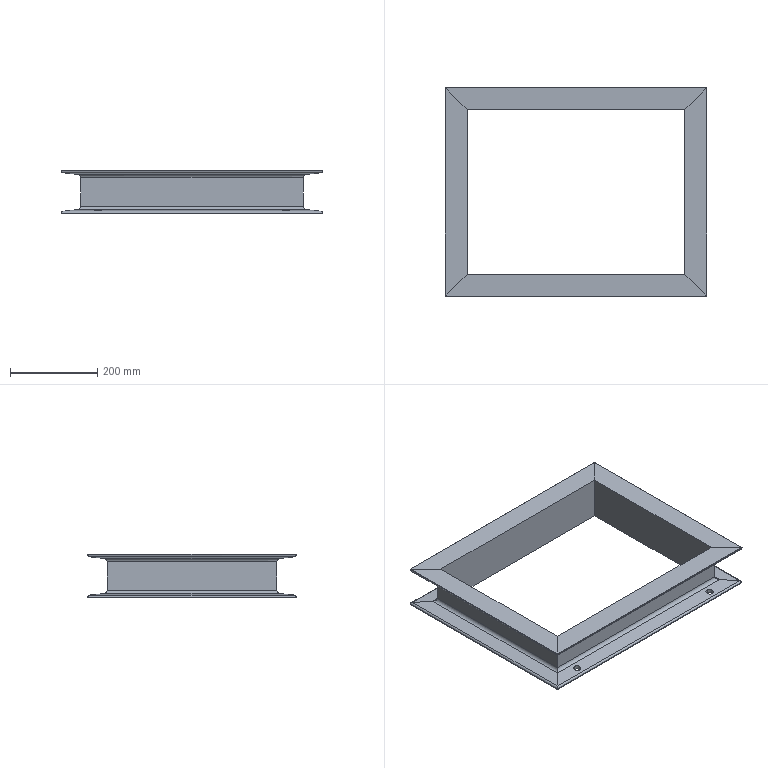Part | SolidWorks | features BaseBody 4, MoveCopyBody 2, MoveFace 2 | 4 solids | 64 faces | box 600 x 478 x 100 mm | volume 2451873 mm3 | plane 40 | cylinder 24 | commonest cylinder face diameters 9 x8 16 x8 17 x8